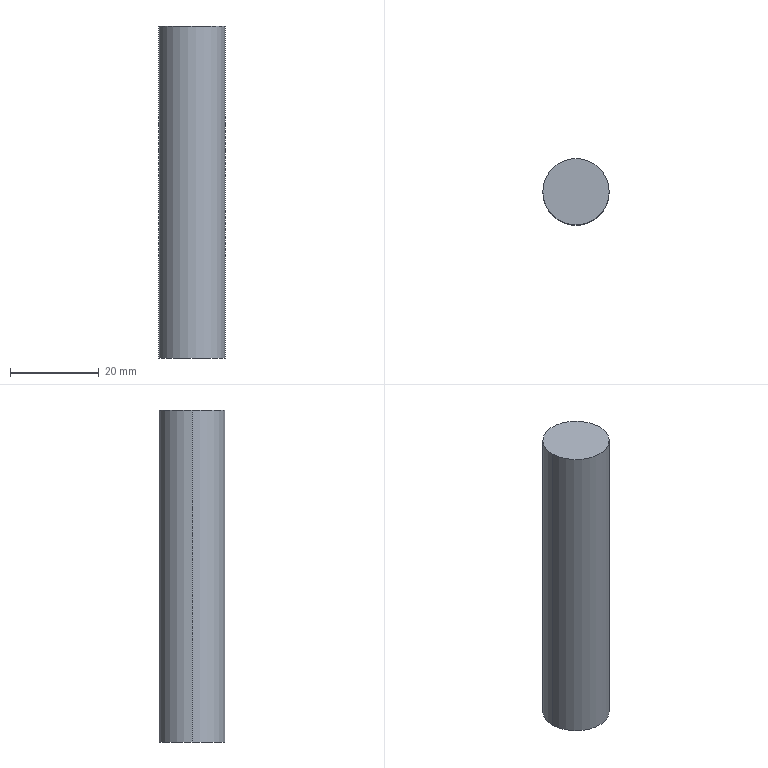Part | SolidWorks | features Revolution 1 | 1 solid | 4 faces | box 15 x 15 x 75 mm | volume 13254 mm3 | cylinder 2 | plane 2 | commonest cylinder face diameters 15 x2
STEP:
#1=CARTESIAN_POINT('',(-7.5,0.,75.));
#2=VERTEX_POINT('',#1);
#3=CARTESIAN_POINT('',(7.5,0.,75.));
#4=VERTEX_POINT('',#3);
#5=CARTESIAN_POINT('',(0.,0.,75.));
#6=DIRECTION('',(0.,0.,-1.));
#7=DIRECTION('',(-1.,0.,0.));
#8=AXIS2_PLACEMENT_3D('',#5,#6,#7);
#9=CIRCLE('',#8,7.5);
#10=EDGE_CURVE('',#2,#4,#9,.T.);
#11=ORIENTED_EDGE('',*,*,#10,.T.);
#12=CARTESIAN_POINT('',(7.5,0.,0.));
#13=VERTEX_POINT('',#12);
#14=CARTESIAN_POINT('',(7.5,0.,75.));
#15=DIRECTION('',(0.,0.,-1.));
#16=VECTOR('',#15,1000.);
#17=LINE('',#14,#16);
#18=EDGE_CURVE('',#4,#13,#17,.T.);
#19=ORIENTED_EDGE('',*,*,#18,.T.);
#20=CARTESIAN_POINT('',(-7.5,0.,0.));
#21=VERTEX_POINT('',#20);
#22=CARTESIAN_POINT('',(0.,0.,0.));
#23=DIRECTION('',(0.,0.,-1.));
#24=DIRECTION('',(-1.,0.,0.));
#25=AXIS2_PLACEMENT_3D('',#22,#23,#24);
#26=CIRCLE('',#25,7.5);
#27=EDGE_CURVE('',#21,#13,#26,.T.);
#28=ORIENTED_EDGE('',*,*,#27,.F.);
#29=CARTESIAN_POINT('',(-7.5,0.,75.));
#30=DIRECTION('',(0.,0.,-1.));
#31=VECTOR('',#30,1000.);
#32=LINE('',#29,#31);
#33=EDGE_CURVE('',#2,#21,#32,.T.);
#34=ORIENTED_EDGE('',*,*,#33,.F.);
#35=EDGE_LOOP('',(#11,#19,#28,#34));
#36=FACE_OUTER_BOUND('',#35,.T.);
#37=CARTESIAN_POINT('',(0.,0.,75.));
#38=DIRECTION('',(0.,0.,-1.));
#39=DIRECTION('',(-1.,0.,0.));
#40=AXIS2_PLACEMENT_3D('',#37,#38,#39);
#41=CYLINDRICAL_SURFACE('',#40,7.5);
#42=ADVANCED_FACE('',(#36),#41,.T.);
#43=ORIENTED_EDGE('',*,*,#18,.F.);
#44=CARTESIAN_POINT('',(0.,0.,75.));
#45=DIRECTION('',(0.,0.,-1.));
#46=DIRECTION('',(-1.,0.,0.));
#47=AXIS2_PLACEMENT_3D('',#44,#45,#46);
#48=CIRCLE('',#47,7.5);
#49=EDGE_CURVE('',#4,#2,#48,.T.);
#50=ORIENTED_EDGE('',*,*,#49,.T.);
#51=ORIENTED_EDGE('',*,*,#33,.T.);
#52=CARTESIAN_POINT('',(0.,0.,0.));
#53=DIRECTION('',(0.,0.,-1.));
#54=DIRECTION('',(-1.,0.,0.));
#55=AXIS2_PLACEMENT_3D('',#52,#53,#54);
#56=CIRCLE('',#55,7.5);
#57=EDGE_CURVE('',#13,#21,#56,.T.);
#58=ORIENTED_EDGE('',*,*,#57,.F.);
#59=EDGE_LOOP('',(#43,#50,#51,#58));
#60=FACE_OUTER_BOUND('',#59,.T.);
#61=CARTESIAN_POINT('',(0.,0.,75.));
#62=DIRECTION('',(0.,0.,-1.));
#63=DIRECTION('',(-1.,0.,0.));
#64=AXIS2_PLACEMENT_3D('',#61,#62,#63);
#65=CYLINDRICAL_SURFACE('',#64,7.5);
#66=ADVANCED_FACE('',(#60),#65,.T.);
#67=ORIENTED_EDGE('',*,*,#10,.F.);
#68=ORIENTED_EDGE('',*,*,#49,.F.);
#69=EDGE_LOOP('',(#67,#68));
#70=FACE_OUTER_BOUND('',#69,.T.);
#71=CARTESIAN_POINT('',(7.5,0.,75.));
#72=DIRECTION('',(0.,0.,1.));
#73=DIRECTION('',(1.,0.,0.));
#74=AXIS2_PLACEMENT_3D('',#71,#72,#73);
#75=PLANE('',#74);
#76=ADVANCED_FACE('',(#70),#75,.T.);
#77=ORIENTED_EDGE('',*,*,#27,.T.);
#78=ORIENTED_EDGE('',*,*,#57,.T.);
#79=EDGE_LOOP('',(#77,#78));
#80=FACE_OUTER_BOUND('',#79,.T.);
#81=CARTESIAN_POINT('',(0.,0.,0.));
#82=DIRECTION('',(0.,0.,-1.));
#83=DIRECTION('',(-1.,0.,0.));
#84=AXIS2_PLACEMENT_3D('',#81,#82,#83);
#85=PLANE('',#84);
#86=ADVANCED_FACE('',(#80),#85,.T.);
#87=CLOSED_SHELL('',(#42,#66,#76,#86));
#88=MANIFOLD_SOLID_BREP('',#87);
#89=CARTESIAN_POINT('',(0.,0.,0.));
#90=DIRECTION('',(0.,0.,1.));
#91=DIRECTION('',(1.,0.,0.));
#92=AXIS2_PLACEMENT_3D('',#89,#90,#91);
#93=(LENGTH_UNIT()NAMED_UNIT(*)SI_UNIT(.MILLI.,.METRE.));
#94=UNCERTAINTY_MEASURE_WITH_UNIT(LENGTH_MEASURE(0.00001),#93,'','');
#95=(NAMED_UNIT(*)PLANE_ANGLE_UNIT()SI_UNIT($,.RADIAN.));
#96=(NAMED_UNIT(*)SI_UNIT($,.STERADIAN.)SOLID_ANGLE_UNIT());
#97=(GEOMETRIC_REPRESENTATION_CONTEXT(3)GLOBAL_UNCERTAINTY_ASSIGNED_CONTEXT((#94))GLOBAL_UNIT_ASSIGNED_CONTEXT((#93,#95,#96))REPRESENTATION_CONTEXT('',''));
#98=ADVANCED_BREP_SHAPE_REPRESENTATION('',(#88,#92),#97);